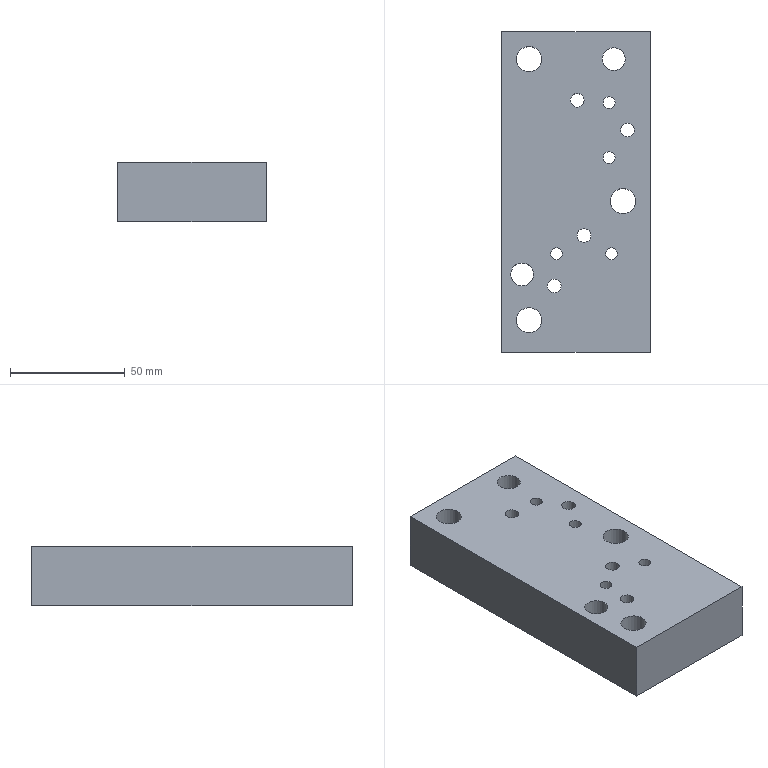Part | STEP file | 103_id38_x_t | 1 solid | 37 faces | box 65 x 140 x 26 mm | volume 209540 mm3 | cylinder 18 | plane 11 | cone 8 | commonest cylinder face diameters 6 x4 8.5 x4 11 x3 17 x3 10 x2 12 x2